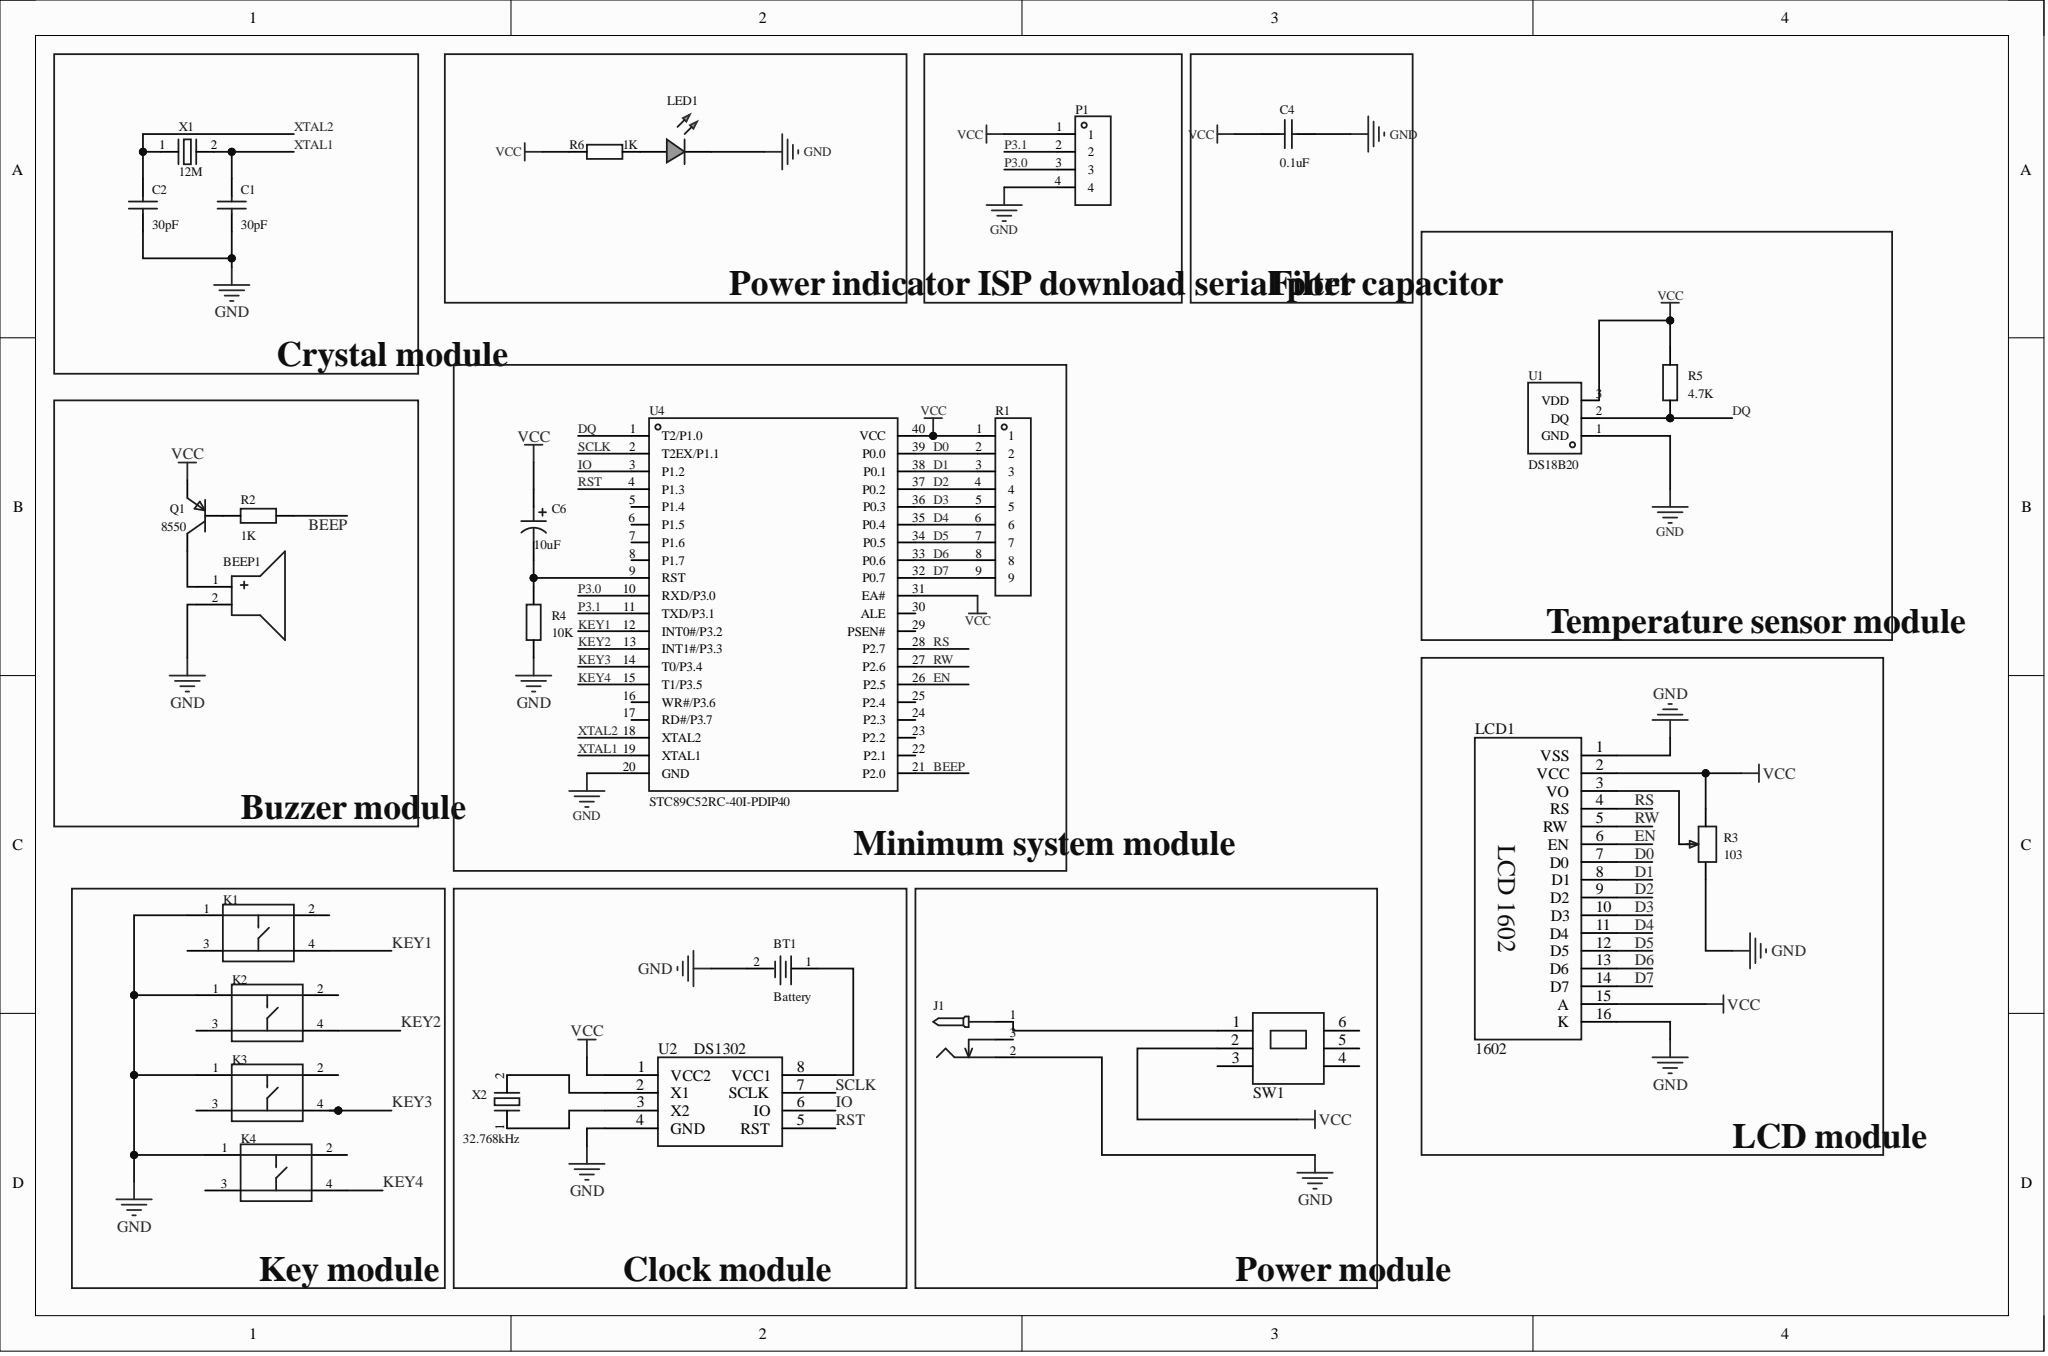Circuit board | Altium Designer | 27 parts | 35 nets
Bill of materials:
Comment,Description,Designator,Footprint,LibRef,Quantity
"","","BEEP1","BUZ-TH_BD12.0-P7.60-D0.6-FD","BZ-D12-L7_6","1"
"Battery","","BT1","BAT-TH_CR2032","Q&J CR2032 20-6*9_C9900112302","1"
"30pF","Capacitance: -; rated voltage: -; temperature coefficient: -;","C1, C2","CAP-TH_L5.0-W4.0-P5.00-D1.0","瓷片电容47PF 3KV","2"
"0.1uF","Capacitance: -; rated voltage: -; temperature coefficient: -;","C4","CAP-TH_L5.0-W4.0-P5.00-D1.0","瓷片电容47PF 3KV","1"
"10uF","","C6","CAP-TH_BD5.0-P2.00-D0.6-FD","10uF/25V-C5X11DIP","1"
"","","J1","DC-005_2.5","DC-005_2.5","1"
"","Circuit structure: SPST; button shape: round button; actuating force: 2.5N; mounting: through-hole; switch length: 6mm; switch width: 6mm; switch height: 5mm; contact current: 50mA; rated voltage: 12V; with light: -; operating life: 10 ten-thousand cycles;","K1, K2, K3, K4","KEY-TH_4P-L6.0-W6.0-P4.50-LS6.50","K2-1102DP-C4SW-04","4"
"1602","","LCD1","HDR-M-2.54_1X16","1602_1","1"
"","","LED1","LED-TH_5mm","LED_TH-G_5mm","1"
"","","P1","HDR-TH_4P-P2.54-V-M","HDR-M_2.54_1x4P","1"
"8550","","Q1","S8550P_TO-92","S8550_TO_PNP","1"
"","","R1","SIP-9_L22.3-W3.2-P2.54_KA2284-SIP-9","HDR-M_2.54-1x9P","1"
"1K","","R2, R6","Res_1/4W","Res_AXIAL-1/4W","2"
"103","","R3","RES-ADJ-SMD_RM065-V1","RM065-V1-103","1"
"10K","","R4","Res_1/4W","Res_AXIAL-1/4W","1"
"4.7K","","R5","Res_1/4W","Res_AXIAL-1/4W","1"
"SWT","","SW1","SW-TH_6P-L8.5-W8.5-P2.50-LS5.5-BL-2","SWT_1","1"
"DS18B20","Detection temperature: -55℃~+125℃; accuracy: ±0.4℃; interface type: single-bus;","U1","TO-92-3_L4.5-W3.5-P1.27-L","DS18B20","1"
"DS1302","","U2","DIP-8_L10.9-W6.4-P2.54-LS7.6-BL","DS1302","1"
"STC89C52RC-40I-PDIP40","CPU core: 51 family; maximum CPU frequency: -;","U4","DIP-40_L52.0-W13.7-P2.54-LS15.2-BL","STC89C52RC-40I-PDIP40","1"
"12M","Crystal type: through-hole crystal; frequency: 16MHz; frequency tolerance at room temperature: ±20ppm; load capacitance: 12pF; frequency stability: ±30ppm;","X1","HC-49S_L11.5-W4.7-P4.88","SWXSBBCVE0-16","1"
"32.768kHz","Frequency: 32.768kHz; frequency tolerance at room temperature: ±20ppm; external load capacitance: 12.5pF; frequency stability (full temperature): -;","X2","CRYSTAL-TH_BD1.4-P0.45-D0.2","AB15T-32.768KHZ","1"
Netlist (Protel format):
[
BEEP1
BUZ-TH_BD12.0-P7.60-D0.6-FD




]
[
BT1
BAT-TH_CR2032
Battery



]
[
C1
CAP-TH_L5.0-W4.0-P5.00-D1.0
30pF



]
[
C2
CAP-TH_L5.0-W4.0-P5.00-D1.0
30pF



]
[
C4
CAP-TH_L5.0-W4.0-P5.00-D1.0
0.1uF



]
[
C6
CAP-TH_BD5.0-P2.00-D0.6-FD
10uF



]
[
J1
DC-005_2.5




]
[
K1
KEY-TH_4P-L6.0-W6.0-P4.50-LS6.50




]
[
K2
KEY-TH_4P-L6.0-W6.0-P4.50-LS6.50




]
[
K3
KEY-TH_4P-L6.0-W6.0-P4.50-LS6.50




]
[
K4
KEY-TH_4P-L6.0-W6.0-P4.50-LS6.50




]
[
LCD1
HDR-M-2.54_1X16
1602



]
[
LED1
LED-TH_5mm




]
[
P1
HDR-TH_4P-P2.54-V-M




]
[
Q1
S8550P_TO-92
8550



]
[
R1
SIP-9_L22.3-W3.2-P2.54_KA2284-SIP-9




]
[
R2
Res_1/4W
1K



]
[
R3
RES-ADJ-SMD_RM065-V1
103



]
[
R4
Res_1/4W
10K



]
[
R5
Res_1/4W
4.7K



]
[
R6
Res_1/4W
1K



]
[
SW1
SW-TH_6P-L8.5-W8.5-P2.50-LS5.5-BL-2
SWT



]
[
U1
TO-92-3_L4.5-W3.5-P1.27-L
DS18B20



]
[
U2
DIP-8_L10.9-W6.4-P2.54-LS7.6-BL
DS1302



]
[
U4
DIP-40_L52.0-W13.7-P2.54-LS15.2-BL
STC89C52RC-40I-PDIP40



]
[
X1
HC-49S_L11.5-W4.7-P4.88
12M



]
[
X2
CRYSTAL-TH_BD1.4-P0.45-D0.2
32.768kHz



]
(
XTAL2
C2-2
U4-18
X1-1
)
(
XTAL1
C1-2
U4-19
X1-2
)
(
VCC
C4-1
C6-1
LCD1-2
LCD1-15
P1-1
Q1-1
R1-1
R3-3
R5-2
R6-1
SW1-2
U1-3
U2-1
U4-31
U4-40
)
(
SCLK
U2-7
U4-2
)
(
RW
LCD1-5
U4-27
)
(
RST
U2-5
U4-4
)
(
RS
LCD1-4
U4-28
)
(
P3.1
P1-2
U4-11
)
(
P3.0
P1-3
U4-10
)
(
NetU2_3
U2-3
X2-1
)
(
NetU2_2
U2-2
X2-2
)
(
NetQ1_2
Q1-2
R2-1
)
(
NetLED1_1
LED1-1
R6-2
)
(
NetLCD1_3
LCD1-3
R3-2
)
(
NetJ1_1
J1-1
SW1-1
)
(
NetC6_2
C6-2
R4-2
U4-9
)
(
NetBT1_1
BT1-1
U2-8
)
(
NetBEEP1_1
BEEP1-1
Q1-3
)
(
KEY4
K4-4
U4-15
)
(
KEY3
K3-4
U4-14
)
(
KEY2
K2-4
U4-13
)
(
KEY1
K1-4
U4-12
)
(
IO
U2-6
U4-3
)
(
GND
BEEP1-2
BT1-2
C1-1
C2-1
C4-2
J1-2
K1-1
K2-1
K3-1
K4-1
LCD1-1
LCD1-16
LED1-2
P1-4
R3-1
R4-1
U1-1
U2-4
U4-20
)
(
EN
LCD1-6
U4-26
)
(
DQ
R5-1
U1-2
U4-1
)
(
D7
LCD1-14
R1-9
U4-32
)
(
D6
LCD1-13
R1-8
U4-33
)
(
D5
LCD1-12
R1-7
U4-34
)
(
D4
LCD1-11
R1-6
U4-35
)
(
D3
LCD1-10
R1-5
U4-36
)
(
D2
LCD1-9
R1-4
U4-37
)
(
D1
LCD1-8
R1-3
U4-38
)
(
D0
LCD1-7
R1-2
U4-39
)
(
BEEP
R2-2
U4-21
)